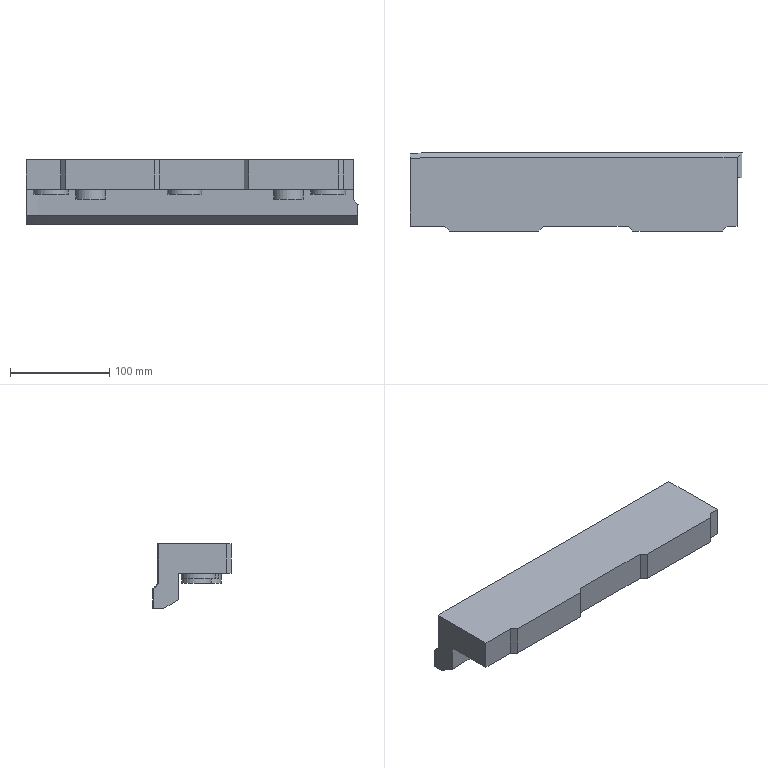Part | NX | features solid 2 | 1 solid | 31 faces | box 335 x 78.909 x 65.334 mm | volume 991028 mm3 | plane 19 | spline 7 | cylinder 5 | commonest cylinder face diameters 35 x3 30 x2